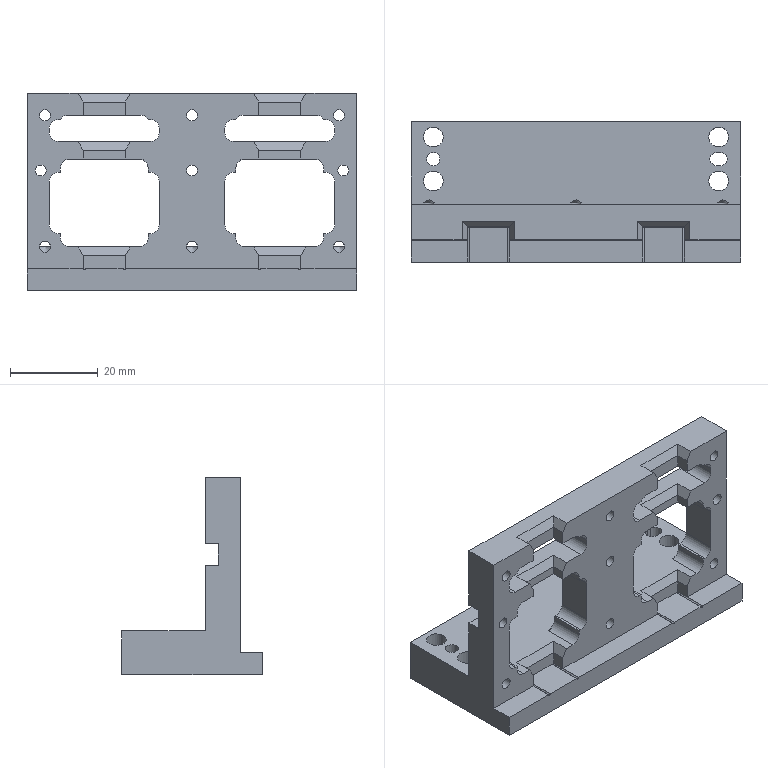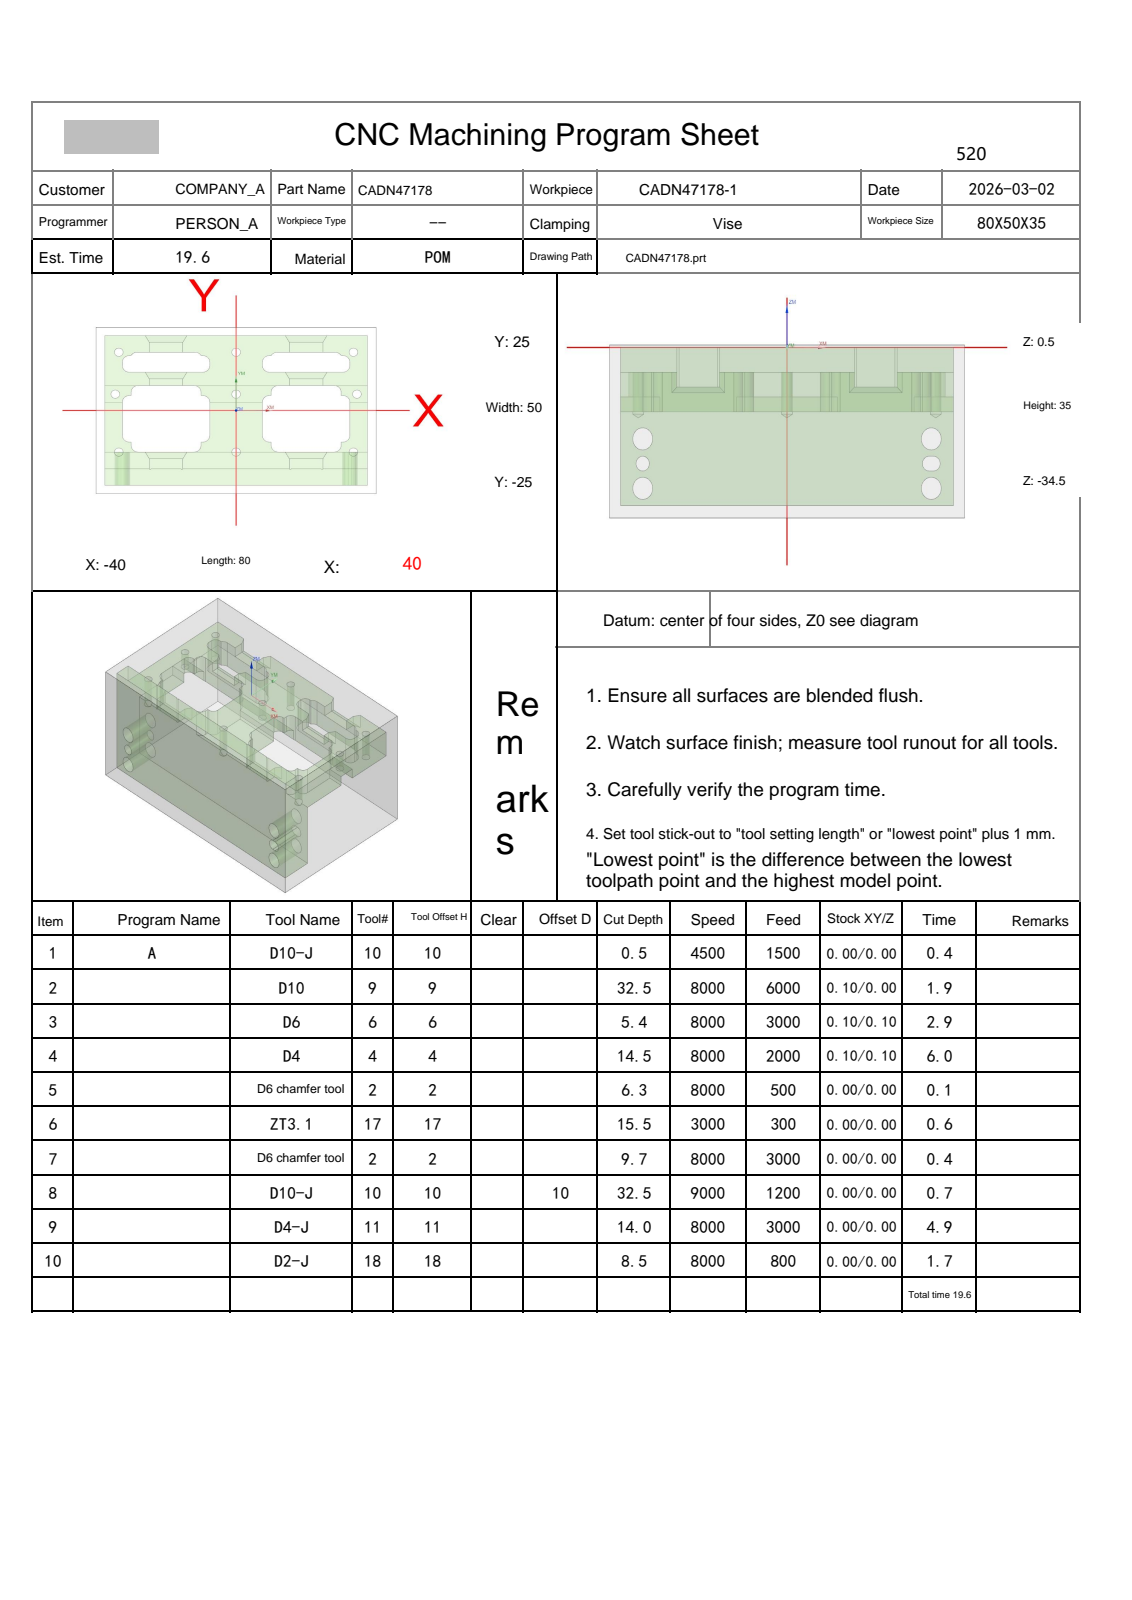NC program | NX | posted by the shop | part box 75 x 32 x 45 mm
Lines 8042 to 8499 of 18359:
N5 T02 M06
(D6 chamfer tool  D=6. R=0. H=02 ce=0.00 di=0.10)
G00 G90 G54 X-33.5 Y-12.5 M03 S8000
G43 H02 Z30.
M08
G98 G81 X-33.5 Y-12.5 Z-5.8 R-4. F500.
X-34.5 Y4.9
X-33.5 Y17.5
X0.0
Y4.9
Y-12.5
X33.5
X34.5 Y4.9
X33.5 Y17.5
G80
G00 Z30.
G91 G28 Z0.0
M05
M09
G91 G28 Z0.0
M01
N6 T17 M06
(ZT3.1 D=3.1 DR_a=118 H=17)
G00 G90 G54 X34.5 Y4.9 M03 S3000
G43 H17 Z30.
M08
G98 G83 X34.5 Y4.9 Z-15. R-4. F300. Q2.
X33.5 Y17.5
X0.0
Y4.9
X-34.5
X-33.5 Y17.5
G80
G00 Z30.
G00 G90 X33.5 Y-12.5 M03 S3000
Z30.
G98 G83 X33.5 Y-12.5 Z-14.5 R-4. F100. Q2.
X0.0
X-33.5
G80
G00 Z30.
G91 G28 Z0.0
M05
M09
G91 G28 Z0.0
M01
N7 T02 M06
(D6 chamfer tool  D=6. R=0. H=02 ce=0.00 di=0.00)
G00 G90 G54 X.25 Y-24.328 M03 S8000
G43 H02 Z30.
M08
Z2.399
G01 Z-1.2 F3000.
G03 X.33 Y-24.028 I-.52 J.3
X.03 Y-23.508 I-.6 J0.0
G01 X0.0 Y-23.5
X-37.5
G02 X-38.5 Y-22.5 I0.0 J1.
G01 Y-17.5
G02 X-37.5 Y-16.5 I1. J0.0
G01 X-24.8
X-24.674 Y-16.508
X-24.55 Y-16.532
X-24.426 Y-16.508
X-24.3 Y-16.5
X-15.7
X-15.574 Y-16.508
X-15.45 Y-16.532
X-15.326 Y-16.508
X-15.2 Y-16.5
X15.2
X15.326 Y-16.508
X15.45 Y-16.532
X15.574 Y-16.508
X15.7 Y-16.5
X24.3
X24.426 Y-16.508
X24.55 Y-16.532
X24.674 Y-16.508
X24.8 Y-16.5
X37.5
G02 X38.5 Y-17.5 I0.0 J-1.
G01 Y-22.5
G02 X37.5 Y-23.5 I-1. J0.0
G01 X0.0
X-.03 Y-23.508
G03 X-.33 Y-24.028 I.3 J-.52
X-.25 Y-24.328 I.6 J0.0
G01 Z2.399
G00 Z30.
X23.11 Y-13.771
Z2.055
G01 Z-6.199
G03 X23.63 Y-14.071 I.52 J.3
X23.93 Y-13.991 I0.0 J.6
G01 X23.952 Y-13.969
X25.089 Y-12.
X25.248 Y-11.793
X25.455 Y-11.634
X25.696 Y-11.534
X25.955 Y-11.5
X28.
G03 X29. Y-10.5 I0.0 J1.
G01 Y-9.5
G02 X30. Y-8.5 I1. J0.0
G01 X30.5
G03 X31.5 Y-7.5 I0.0 J1.
G01 Y2.5
G03 X30.5 Y3.5 I-1. J0.0
G01 X30.
G02 X29. Y4.5 I0.0 J1.
G01 Y5.5
G03 X28. Y6.5 I-1. J0.0
G01 X24.8
G02 X23.8 Y7.5 I0.0 J1.
G01 Y9.5
X23.834 Y9.759
X23.934 Y10.
X25.089 Y12.
X25.248 Y12.207
X25.455 Y12.366
X25.696 Y12.466
X25.955 Y12.5
X30.5
G03 X31.5 Y13.5 I0.0 J1.
G01 Y14.5
G03 X30.5 Y15.5 I-1. J0.0
G01 X30.
X29.741 Y15.534
X29.5 Y15.634
X29.293 Y15.793
X28.975 Y16.207
X28.768 Y16.366
X28.527 Y16.466
X28.268 Y16.5
X24.8
G02 X23.8 Y17.5 I0.0 J1.
G01 Y20.5
X23.834 Y20.759
X23.934 Y21.
X25.089 Y23.
X25.248 Y23.207
X25.455 Y23.366
X25.696 Y23.466
X25.955 Y23.5
X37.5
G02 X38.5 Y22.5 I0.0 J-1.
G01 Y-14.102
X38.506 Y-14.126
G03 X38.922 Y-14.366 I.416 J.24
X39.162 Y-14.301 I0.0 J.48
G01 Z2.055
G00 Z30.
X-16.89 Y-13.771
Z2.055
G01 Z-6.199
G03 X-16.37 Y-14.071 I.52 J.3
X-16.07 Y-13.991 I0.0 J.6
G01 X-16.048 Y-13.969
X-14.911 Y-12.
X-14.752 Y-11.793
X-14.545 Y-11.634
X-14.304 Y-11.534
X-14.045 Y-11.5
X-12.
G03 X-11. Y-10.5 I0.0 J1.
G01 Y-9.5
G02 X-10. Y-8.5 I1. J0.0
G01 X-9.5
G03 X-8.5 Y-7.5 I0.0 J1.
G01 Y2.5
G03 X-9.5 Y3.5 I-1. J0.0
G01 X-10.
G02 X-11. Y4.5 I0.0 J1.
G01 Y5.5
G03 X-12. Y6.5 I-1. J0.0
G01 X-15.2
G02 X-16.2 Y7.5 I0.0 J1.
G01 Y9.5
X-16.166 Y9.759
X-16.066 Y10.
X-14.911 Y12.
X-14.752 Y12.207
X-14.545 Y12.366
X-14.304 Y12.466
X-14.045 Y12.5
X-9.5
G03 X-8.5 Y13.5 I0.0 J1.
G01 Y14.5
G03 X-9.5 Y15.5 I-1. J0.0
G01 X-10.
X-10.259 Y15.534
X-10.5 Y15.634
X-10.707 Y15.793
X-11.025 Y16.207
X-11.232 Y16.366
X-11.473 Y16.466
X-11.732 Y16.5
X-15.2
G02 X-16.2 Y17.5 I0.0 J1.
G01 Y20.5
X-16.166 Y20.759
X-16.066 Y21.
X-14.911 Y23.
X-14.752 Y23.207
X-14.545 Y23.366
X-14.304 Y23.466
X-14.045 Y23.5
X14.045
X14.304 Y23.466
X14.545 Y23.366
X14.752 Y23.207
X14.911 Y23.
X16.066 Y21.
X16.166 Y20.759
X16.2 Y20.5
Y17.5
G02 X15.2 Y16.5 I-1. J0.0
G01 X11.732
X11.473 Y16.466
X11.232 Y16.366
X11.025 Y16.207
X10.707 Y15.793
X10.5 Y15.634
X10.259 Y15.534
X10. Y15.5
X9.5
G03 X8.5 Y14.5 I0.0 J-1.
G01 Y13.5
G03 X9.5 Y12.5 I1. J0.0
G01 X14.045
X14.304 Y12.466
X14.545 Y12.366
X14.752 Y12.207
X14.911 Y12.
X16.066 Y10.
X16.166 Y9.759
X16.2 Y9.5
Y7.5
G02 X15.2 Y6.5 I-1. J0.0
G01 X12.
G03 X11. Y5.5 I0.0 J-1.
G01 Y4.5
G02 X10. Y3.5 I-1. J0.0
G01 X9.5
G03 X8.5 Y2.5 I0.0 J-1.
G01 Y-7.5
G03 X9.5 Y-8.5 I1. J0.0
G01 X10.
G02 X11. Y-9.5 I0.0 J-1.
G01 Y-10.5
G03 X12. Y-11.5 I1. J0.0
G01 X14.045
X14.304 Y-11.534
X14.545 Y-11.634
X14.752 Y-11.793
X14.911 Y-12.
X16.048 Y-13.969
X16.07 Y-13.991
G03 X16.37 Y-14.071 I.3 J.52
X16.89 Y-13.771 I0.0 J.6
G01 Z2.055
G00 Z30.
X-39.162 Y-14.301
Z2.055
G01 Z-6.199
G03 X-38.922 Y-14.366 I.24 J.416
X-38.506 Y-14.126 I0.0 J.48
G01 X-38.5 Y-14.102
Y22.5
G02 X-37.5 Y23.5 I1. J0.0
G01 X-25.955
X-25.696 Y23.466
X-25.455 Y23.366
X-25.248 Y23.207
X-25.089 Y23.
X-23.934 Y21.
X-23.834 Y20.759
X-23.8 Y20.5
Y17.5
G02 X-24.8 Y16.5 I-1. J0.0
G01 X-28.268
X-28.527 Y16.466
X-28.768 Y16.366
X-28.975 Y16.207
X-29.293 Y15.793
X-29.5 Y15.634
X-29.741 Y15.534
X-30. Y15.5
X-30.5
G03 X-31.5 Y14.5 I0.0 J-1.
G01 Y13.5
G03 X-30.5 Y12.5 I1. J0.0
G01 X-25.955
X-25.696 Y12.466
X-25.455 Y12.366
X-25.248 Y12.207
X-25.089 Y12.
X-23.934 Y10.
X-23.834 Y9.759
X-23.8 Y9.5
Y7.5
G02 X-24.8 Y6.5 I-1. J0.0
G01 X-28.
G03 X-29. Y5.5 I0.0 J-1.
G01 Y4.5
G02 X-30. Y3.5 I-1. J0.0
G01 X-30.5
G03 X-31.5 Y2.5 I0.0 J-1.
G01 Y-7.5
G03 X-30.5 Y-8.5 I1. J0.0
G01 X-30.
G02 X-29. Y-9.5 I0.0 J-1.
G01 Y-10.5
G03 X-28. Y-11.5 I1. J0.0
G01 X-25.955
X-25.696 Y-11.534
X-25.455 Y-11.634
X-25.248 Y-11.793
X-25.089 Y-12.
X-23.952 Y-13.969
X-23.93 Y-13.991
G03 X-23.63 Y-14.071 I.3 J.52
X-23.11 Y-13.771 I0.0 J.6
G01 Z2.055
G00 Z30.
X-18.4 Y15.921
Z-2.945
G01 Z-9.199
G03 X-18.344 Y16.131 I-.364 J.21
X-18.554 Y16.494 I-.42 J0.0
G01 X-18.575 Y16.5
X-21.425
X-21.446 Y16.494
G03 X-21.656 Y16.131 I.21 J-.364
X-21.6 Y15.921 I.42 J0.0
G01 Z-2.945
G00 Z-1.699
X-18.4 Y5.921
Z-2.945
G01 Z-9.199
G03 X-18.344 Y6.131 I-.364 J.21
X-18.554 Y6.494 I-.42 J0.0
G01 X-18.575 Y6.5
X-21.425
X-21.446 Y6.494
G03 X-21.656 Y6.131 I.21 J-.364
X-21.6 Y5.921 I.42 J0.0
G01 Z-2.945
G00 Z30.
X21.6
Z-2.945
G01 Z-9.199
G03 X21.656 Y6.131 I-.364 J.21
X21.446 Y6.494 I-.42 J0.0
G01 X21.425 Y6.5
X18.575
X18.554 Y6.494
G03 X18.344 Y6.131 I.21 J-.364
X18.4 Y5.921 I.42 J0.0
G01 Z-2.945
G00 Z-1.699
X21.6 Y15.921
Z-2.945
G01 Z-9.199
G03 X21.656 Y16.131 I-.364 J.21
X21.446 Y16.494 I-.42 J0.0
G01 X21.425 Y16.5
X18.575
X18.554 Y16.494
G03 X18.344 Y16.131 I.21 J-.364
X18.4 Y15.921 I.42 J0.0
G01 Z-2.945
G00 Z30.
G00 G90 X-33.5 Y-12.5 M03 S8000
Z30.
G98 G81 X-33.5 Y-12.5 Z-6.75 R-2. F500.
X-34.5 Y4.9
X-33.5 Y17.5
X0.0
Y4.9
Y-12.5
X33.5
X34.5 Y4.9
X33.5 Y17.5
G80
G00 Z30.
G91 G28 Z0.0
M05
M09
G91 G28 Z0.0
M01
N8 T10 M06
(D10-J  D=10. R=0. H=10 ce=0.00 di=0.00)
G00 G90 G54 X-38.513 Y28.616 M03 S9000
G43 H10 Z30.
M08
Z-10.167
G01 Z-10.667 F1200.
G41 D10
X-38.497 Y28.417
G03 X-37.5 Y27.5 I.997 J.083
G01 X37.5
G02 X42.5 Y22.5 I0.0 J-5.
G01 Y-22.5
G02 X37.5 Y-27.5 I-5. J0.0
G01 X-37.5
G02 X-42.5 Y-22.5 I0.0 J5.
G01 Y22.5
G02 X-37.5 Y27.5 I5. J0.0
G01 X-37.
G03 X-36. Y28.5 I0.0 J1.
G01 G40 Y28.7
Z-10.167
G00 Z30.
X-38.513 Y28.616
Z-20.833
G01 Z-21.333
G41 D10
X-38.497 Y28.417
G03 X-37.5 Y27.5 I.997 J.083
G01 X37.5
G02 X42.5 Y22.5 I0.0 J-5.
G01 Y-22.5
G02 X37.5 Y-27.5 I-5. J0.0
G01 X-37.5
G02 X-42.5 Y-22.5 I0.0 J5.
G01 Y22.5
G02 X-37.5 Y27.5 I5. J0.0
G01 X-37.
G03 X-36. Y28.5 I0.0 J1.
G01 G40 Y28.7
Z-20.833
G00 Z30.
X-38.513 Y28.616
Z-31.5
G01 Z-32.
G41 D10
X-38.497 Y28.417
G03 X-37.5 Y27.5 I.997 J.083
G01 X37.5
G02 X42.5 Y22.5 I0.0 J-5.
G01 Y-22.5
G02 X37.5 Y-27.5 I-5. J0.0
G01 X-37.5
G02 X-42.5 Y-22.5 I0.0 J5.
G01 Y22.5
G02 X-37.5 Y27.5 I5. J0.0
G01 X-37.
G03 X-36. Y28.5 I0.0 J1.
G01 G40 Y28.7
Z-31.5
G00 Z30.
G91 G28 Z0.0
M05
M09
G91 G28 Z0.0
M01